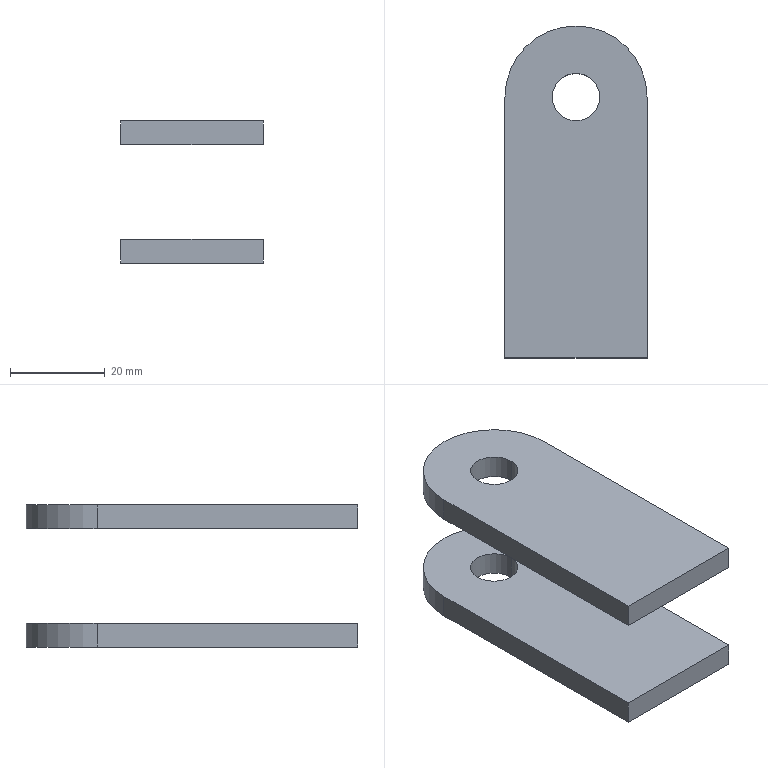Part | SolidWorks | 2 solids | 16 faces | box 30 x 70 x 30 mm | volume 19249 mm3 | plane 10 | cylinder 6 | commonest cylinder face diameters 10 x4 30 x2